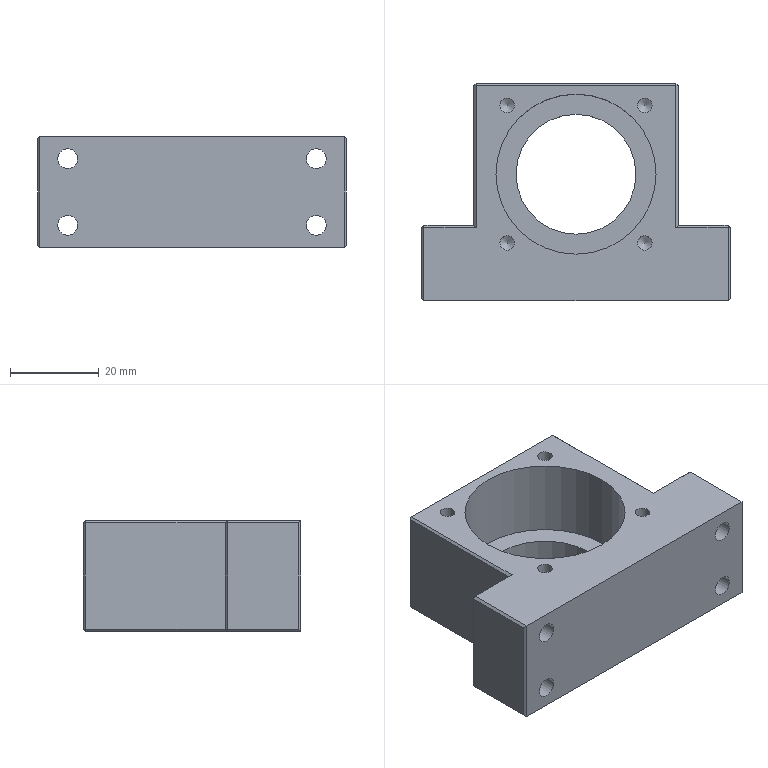Part | STEP file | 1 solid | 61 faces | box 69.5 x 49 x 25 mm | volume 41553 mm3 | plane 43 | cylinder 14 | cone 4 | commonest cylinder face diameters 3.3 x4 4.5 x4 8 x4 27 x1 36.05 x1